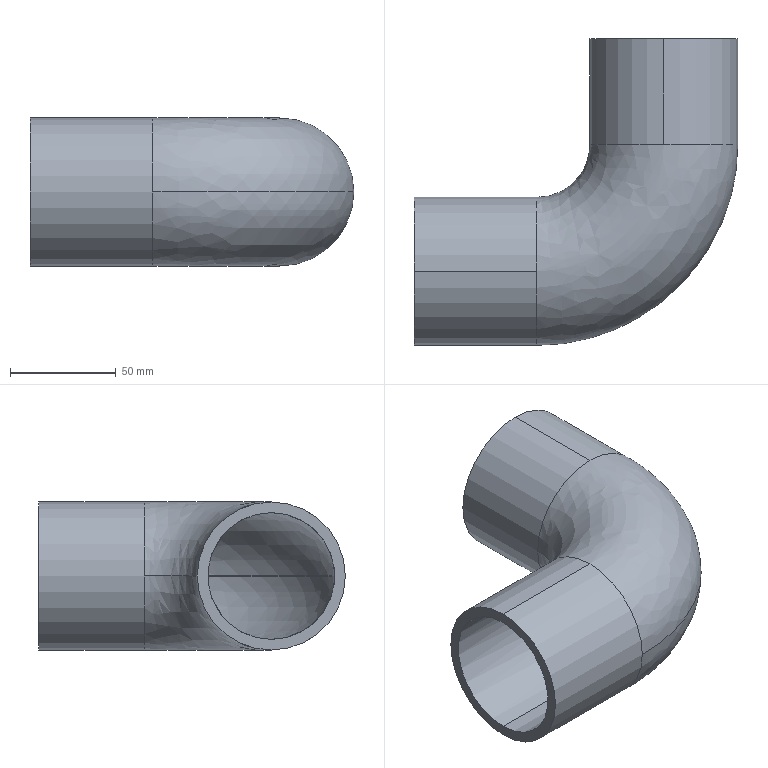Part | SolidWorks | features BaseBody 1 | 1 solid | 15 faces | box 153.045 x 145 x 70 mm | volume 206542 mm3 | cylinder 8 | spline 5 | plane 2 | commonest cylinder face diameters 60 x4 70 x4
STEP:
#1=CARTESIAN_POINT('',(58.045,0.,-35.));
#2=VERTEX_POINT('',#1);
#3=CARTESIAN_POINT('',(58.045,35.,-0.004506));
#4=VERTEX_POINT('',#3);
#5=CARTESIAN_POINT('',(58.045,0.,0.));
#6=DIRECTION('',(1.,0.,0.));
#7=DIRECTION('',(0.,-1.,0.));
#8=AXIS2_PLACEMENT_3D('',#5,#6,#7);
#9=CIRCLE('',#8,35.);
#10=EDGE_CURVE('',#2,#4,#9,.T.);
#11=ORIENTED_EDGE('',*,*,#10,.F.);
#12=CARTESIAN_POINT('',(0.,0.,-35.));
#13=VERTEX_POINT('',#12);
#14=CARTESIAN_POINT('',(58.045,0.,-35.));
#15=DIRECTION('',(-1.,0.,0.));
#16=VECTOR('',#15,1000.);
#17=LINE('',#14,#16);
#18=EDGE_CURVE('',#2,#13,#17,.T.);
#19=ORIENTED_EDGE('',*,*,#18,.T.);
#20=CARTESIAN_POINT('',(0.,0.,35.));
#21=VERTEX_POINT('',#20);
#22=CARTESIAN_POINT('',(0.,0.,0.));
#23=DIRECTION('',(1.,0.,0.));
#24=DIRECTION('',(0.,0.,1.));
#25=AXIS2_PLACEMENT_3D('',#22,#23,#24);
#26=CIRCLE('',#25,35.);
#27=EDGE_CURVE('',#13,#21,#26,.T.);
#28=ORIENTED_EDGE('',*,*,#27,.T.);
#29=CARTESIAN_POINT('',(58.045,0.,35.));
#30=VERTEX_POINT('',#29);
#31=CARTESIAN_POINT('',(58.045,0.,35.));
#32=DIRECTION('',(-1.,0.,0.));
#33=VECTOR('',#32,1000.);
#34=LINE('',#31,#33);
#35=EDGE_CURVE('',#30,#21,#34,.T.);
#36=ORIENTED_EDGE('',*,*,#35,.F.);
#37=CARTESIAN_POINT('',(58.045,0.,0.));
#38=DIRECTION('',(-1.,0.,0.));
#39=DIRECTION('',(0.,0.,1.));
#40=AXIS2_PLACEMENT_3D('',#37,#38,#39);
#41=CIRCLE('',#40,35.);
#42=EDGE_CURVE('',#30,#4,#41,.T.);
#43=ORIENTED_EDGE('',*,*,#42,.T.);
#44=EDGE_LOOP('',(#11,#19,#28,#36,#43));
#45=FACE_OUTER_BOUND('',#44,.T.);
#46=CARTESIAN_POINT('',(58.045,0.,0.));
#47=DIRECTION('',(-1.,0.,0.));
#48=DIRECTION('',(0.,0.,1.));
#49=AXIS2_PLACEMENT_3D('',#46,#47,#48);
#50=CYLINDRICAL_SURFACE('',#49,35.);
#51=ADVANCED_FACE('',(#45),#50,.T.);
#52=CARTESIAN_POINT('',(118.045,60.,-35.));
#53=VERTEX_POINT('',#52);
#54=CARTESIAN_POINT('',(153.045,60.,0.000000001));
#55=VERTEX_POINT('',#54);
#56=CARTESIAN_POINT('',(118.045,60.,0.));
#57=DIRECTION('',(0.,-1.,0.));
#58=DIRECTION('',(1.,0.,0.));
#59=AXIS2_PLACEMENT_3D('',#56,#57,#58);
#60=CIRCLE('',#59,35.);
#61=EDGE_CURVE('',#53,#55,#60,.T.);
#62=ORIENTED_EDGE('',*,*,#61,.F.);
#63=CARTESIAN_POINT('',(118.045,110.,-35.));
#64=VERTEX_POINT('',#63);
#65=CARTESIAN_POINT('',(118.045,60.,-35.));
#66=DIRECTION('',(0.,1.,0.));
#67=VECTOR('',#66,1000.);
#68=LINE('',#65,#67);
#69=EDGE_CURVE('',#53,#64,#68,.T.);
#70=ORIENTED_EDGE('',*,*,#69,.T.);
#71=CARTESIAN_POINT('',(118.045,110.,35.));
#72=VERTEX_POINT('',#71);
#73=CARTESIAN_POINT('',(118.045,110.,0.));
#74=DIRECTION('',(0.,-1.,0.));
#75=DIRECTION('',(0.,0.,1.));
#76=AXIS2_PLACEMENT_3D('',#73,#74,#75);
#77=CIRCLE('',#76,35.);
#78=EDGE_CURVE('',#64,#72,#77,.T.);
#79=ORIENTED_EDGE('',*,*,#78,.T.);
#80=CARTESIAN_POINT('',(118.045,60.,35.));
#81=VERTEX_POINT('',#80);
#82=CARTESIAN_POINT('',(118.045,60.,35.));
#83=DIRECTION('',(0.,1.,0.));
#84=VECTOR('',#83,1000.);
#85=LINE('',#82,#84);
#86=EDGE_CURVE('',#81,#72,#85,.T.);
#87=ORIENTED_EDGE('',*,*,#86,.F.);
#88=CARTESIAN_POINT('',(118.045,60.,0.000000001));
#89=DIRECTION('',(0.,-1.,0.));
#90=DIRECTION('',(1.,0.,0.));
#91=AXIS2_PLACEMENT_3D('',#88,#89,#90);
#92=CIRCLE('',#91,35.);
#93=EDGE_CURVE('',#55,#81,#92,.T.);
#94=ORIENTED_EDGE('',*,*,#93,.F.);
#95=EDGE_LOOP('',(#62,#70,#79,#87,#94));
#96=FACE_OUTER_BOUND('',#95,.T.);
#97=CARTESIAN_POINT('',(118.045,60.,0.));
#98=DIRECTION('',(0.,1.,0.));
#99=DIRECTION('',(0.,0.,1.));
#100=AXIS2_PLACEMENT_3D('',#97,#98,#99);
#101=CYLINDRICAL_SURFACE('',#100,35.);
#102=ADVANCED_FACE('',(#96),#101,.T.);
#103=CARTESIAN_POINT('',(58.045,0.,-30.));
#104=VERTEX_POINT('',#103);
#105=CARTESIAN_POINT('',(58.045,-30.,-0.000000002));
#106=VERTEX_POINT('',#105);
#107=CARTESIAN_POINT('',(58.045,0.,0.));
#108=DIRECTION('',(-1.,0.,0.));
#109=DIRECTION('',(0.,0.,1.));
#110=AXIS2_PLACEMENT_3D('',#107,#108,#109);
#111=CIRCLE('',#110,30.);
#112=EDGE_CURVE('',#104,#106,#111,.T.);
#113=ORIENTED_EDGE('',*,*,#112,.F.);
#114=CARTESIAN_POINT('',(0.,0.,-30.));
#115=VERTEX_POINT('',#114);
#116=CARTESIAN_POINT('',(58.045,0.,-30.));
#117=DIRECTION('',(-1.,0.,0.));
#118=VECTOR('',#117,1000.);
#119=LINE('',#116,#118);
#120=EDGE_CURVE('',#104,#115,#119,.T.);
#121=ORIENTED_EDGE('',*,*,#120,.T.);
#122=CARTESIAN_POINT('',(0.,0.,30.));
#123=VERTEX_POINT('',#122);
#124=CARTESIAN_POINT('',(0.,0.,0.));
#125=DIRECTION('',(-1.,0.,0.));
#126=DIRECTION('',(0.,0.,1.));
#127=AXIS2_PLACEMENT_3D('',#124,#125,#126);
#128=CIRCLE('',#127,30.);
#129=EDGE_CURVE('',#115,#123,#128,.T.);
#130=ORIENTED_EDGE('',*,*,#129,.T.);
#131=CARTESIAN_POINT('',(58.045,0.,30.));
#132=VERTEX_POINT('',#131);
#133=CARTESIAN_POINT('',(58.045,0.,30.));
#134=DIRECTION('',(-1.,0.,0.));
#135=VECTOR('',#134,1000.);
#136=LINE('',#133,#135);
#137=EDGE_CURVE('',#132,#123,#136,.T.);
#138=ORIENTED_EDGE('',*,*,#137,.F.);
#139=CARTESIAN_POINT('',(58.045,-30.,0.0003745));
#140=VERTEX_POINT('',#139);
#141=CARTESIAN_POINT('',(58.045,0.,0.));
#142=DIRECTION('',(-1.,0.,0.));
#143=DIRECTION('',(0.,0.,1.));
#144=AXIS2_PLACEMENT_3D('',#141,#142,#143);
#145=CIRCLE('',#144,30.);
#146=EDGE_CURVE('',#140,#132,#145,.T.);
#147=ORIENTED_EDGE('',*,*,#146,.F.);
#148=CARTESIAN_POINT('',(58.045,0.,0.));
#149=DIRECTION('',(-1.,0.,0.));
#150=DIRECTION('',(0.,0.,1.));
#151=AXIS2_PLACEMENT_3D('',#148,#149,#150);
#152=CIRCLE('',#151,30.);
#153=EDGE_CURVE('',#106,#140,#152,.T.);
#154=ORIENTED_EDGE('',*,*,#153,.F.);
#155=EDGE_LOOP('',(#113,#121,#130,#138,#147,#154));
#156=FACE_OUTER_BOUND('',#155,.T.);
#157=CARTESIAN_POINT('',(58.045,0.,0.));
#158=DIRECTION('',(-1.,0.,0.));
#159=DIRECTION('',(0.,0.,1.));
#160=AXIS2_PLACEMENT_3D('',#157,#158,#159);
#161=CYLINDRICAL_SURFACE('',#160,30.);
#162=ADVANCED_FACE('',(#156),#161,.F.);
#163=CARTESIAN_POINT('',(118.045,60.,-30.));
#164=VERTEX_POINT('',#163);
#165=CARTESIAN_POINT('',(88.045,60.,-0.000000012));
#166=VERTEX_POINT('',#165);
#167=CARTESIAN_POINT('',(118.045,60.,0.));
#168=DIRECTION('',(0.,1.,0.));
#169=DIRECTION('',(0.,0.,1.));
#170=AXIS2_PLACEMENT_3D('',#167,#168,#169);
#171=CIRCLE('',#170,30.);
#172=EDGE_CURVE('',#164,#166,#171,.T.);
#173=ORIENTED_EDGE('',*,*,#172,.F.);
#174=CARTESIAN_POINT('',(118.045,110.,-30.));
#175=VERTEX_POINT('',#174);
#176=CARTESIAN_POINT('',(118.045,60.,-30.));
#177=DIRECTION('',(0.,1.,0.));
#178=VECTOR('',#177,1000.);
#179=LINE('',#176,#178);
#180=EDGE_CURVE('',#164,#175,#179,.T.);
#181=ORIENTED_EDGE('',*,*,#180,.T.);
#182=CARTESIAN_POINT('',(118.045,110.,30.));
#183=VERTEX_POINT('',#182);
#184=CARTESIAN_POINT('',(118.045,110.,0.));
#185=DIRECTION('',(0.,-1.,0.));
#186=DIRECTION('',(0.,0.,1.));
#187=AXIS2_PLACEMENT_3D('',#184,#185,#186);
#188=CIRCLE('',#187,30.);
#189=EDGE_CURVE('',#183,#175,#188,.T.);
#190=ORIENTED_EDGE('',*,*,#189,.F.);
#191=CARTESIAN_POINT('',(118.045,60.,30.));
#192=VERTEX_POINT('',#191);
#193=CARTESIAN_POINT('',(118.045,60.,30.));
#194=DIRECTION('',(0.,1.,0.));
#195=VECTOR('',#194,1000.);
#196=LINE('',#193,#195);
#197=EDGE_CURVE('',#192,#183,#196,.T.);
#198=ORIENTED_EDGE('',*,*,#197,.F.);
#199=CARTESIAN_POINT('',(118.045,60.,0.));
#200=DIRECTION('',(0.,1.,0.));
#201=DIRECTION('',(0.,0.,1.));
#202=AXIS2_PLACEMENT_3D('',#199,#200,#201);
#203=CIRCLE('',#202,30.);
#204=EDGE_CURVE('',#166,#192,#203,.T.);
#205=ORIENTED_EDGE('',*,*,#204,.F.);
#206=EDGE_LOOP('',(#173,#181,#190,#198,#205));
#207=FACE_OUTER_BOUND('',#206,.T.);
#208=CARTESIAN_POINT('',(118.045,60.,0.));
#209=DIRECTION('',(0.,1.,0.));
#210=DIRECTION('',(0.,0.,1.));
#211=AXIS2_PLACEMENT_3D('',#208,#209,#210);
#212=CYLINDRICAL_SURFACE('',#211,30.);
#213=ADVANCED_FACE('',(#207),#212,.F.);
#214=CARTESIAN_POINT('',(58.045,30.,-0.000000006));
#215=VERTEX_POINT('',#214);
#216=CARTESIAN_POINT('',(58.045,0.,0.));
#217=DIRECTION('',(-1.,0.,0.));
#218=DIRECTION('',(0.,0.,1.));
#219=AXIS2_PLACEMENT_3D('',#216,#217,#218);
#220=CIRCLE('',#219,30.);
#221=EDGE_CURVE('',#215,#104,#220,.T.);
#222=ORIENTED_EDGE('',*,*,#221,.T.);
#223=ORIENTED_EDGE('',*,*,#112,.T.);
#224=CARTESIAN_POINT('',(148.045,60.,-0.000000002));
#225=VERTEX_POINT('',#224);
#226=CARTESIAN_POINT('',(58.045,60.,-0.000000004));
#227=DIRECTION('',(0.,0.,1.));
#228=DIRECTION('',(0.,-1.,0.));
#229=AXIS2_PLACEMENT_3D('',#226,#227,#228);
#230=CIRCLE('',#229,90.);
#231=EDGE_CURVE('',#106,#225,#230,.T.);
#232=ORIENTED_EDGE('',*,*,#231,.T.);
#233=CARTESIAN_POINT('',(118.045,60.,0.));
#234=DIRECTION('',(0.,1.,0.));
#235=DIRECTION('',(0.,0.,1.));
#236=AXIS2_PLACEMENT_3D('',#233,#234,#235);
#237=CIRCLE('',#236,30.);
#238=EDGE_CURVE('',#225,#164,#237,.T.);
#239=ORIENTED_EDGE('',*,*,#238,.T.);
#240=ORIENTED_EDGE('',*,*,#172,.T.);
#241=CARTESIAN_POINT('',(58.045,30.,-0.000000006));
#242=CARTESIAN_POINT('',(60.009,30.,-0.0002528));
#243=CARTESIAN_POINT('',(61.972,30.193,-0.000474));
#244=CARTESIAN_POINT('',(65.823,30.96,-0.0008532));
#245=CARTESIAN_POINT('',(67.711,31.532,-0.001011));
#246=CARTESIAN_POINT('',(71.34,33.035,-0.001264));
#247=CARTESIAN_POINT('',(73.08,33.965,-0.001359));
#248=CARTESIAN_POINT('',(76.345,36.147,-0.001485));
#249=CARTESIAN_POINT('',(77.87,37.398,-0.001517));
#250=CARTESIAN_POINT('',(80.647,40.175,-0.001517));
#251=CARTESIAN_POINT('',(81.898,41.7,-0.001485));
#252=CARTESIAN_POINT('',(84.08,44.965,-0.001359));
#253=CARTESIAN_POINT('',(85.01,46.705,-0.001264));
#254=CARTESIAN_POINT('',(86.513,50.334,-0.001011));
#255=CARTESIAN_POINT('',(87.086,52.222,-0.0008532));
#256=CARTESIAN_POINT('',(87.852,56.073,-0.000474));
#257=CARTESIAN_POINT('',(88.045,58.037,-0.0002528));
#258=CARTESIAN_POINT('',(88.045,60.,-0.000000012));
#259=B_SPLINE_CURVE_WITH_KNOTS('',3,(#241,#242,#243,#244,#245,#246,#247,#248,#249,#250,#251,#252,#253,#254,#255,#256,#257,#258),.UNSPECIFIED.,.F.,.F.,(4,2,2,2,2,2,2,2,4),(0.,0.125,0.25,0.375,0.5,0.625,0.75,0.875,1.),.UNSPECIFIED.);
#260=EDGE_CURVE('',#215,#166,#259,.T.);
#261=ORIENTED_EDGE('',*,*,#260,.F.);
#262=EDGE_LOOP('',(#222,#223,#232,#239,#240,#261));
#263=FACE_OUTER_BOUND('',#262,.T.);
#264=CARTESIAN_POINT('',(58.045,-30.,-0.000000002));
#265=CARTESIAN_POINT('',(110.766,-30.,-0.000000001));
#266=CARTESIAN_POINT('',(148.045,7.279,-0.000000001));
#267=CARTESIAN_POINT('',(148.045,60.,-0.000000002));
#268=CARTESIAN_POINT('',(58.045,-30.,-17.705));
#269=CARTESIAN_POINT('',(110.766,-30.,-17.705));
#270=CARTESIAN_POINT('',(148.045,7.279,-17.705));
#271=CARTESIAN_POINT('',(148.045,60.,-17.705));
#272=CARTESIAN_POINT('',(58.045,-17.422,-30.166));
#273=CARTESIAN_POINT('',(103.398,-17.422,-30.166));
#274=CARTESIAN_POINT('',(135.467,14.647,-30.166));
#275=CARTESIAN_POINT('',(135.467,60.,-30.166));
#276=CARTESIAN_POINT('',(58.045,0.2827,-29.999));
#277=CARTESIAN_POINT('',(93.027,0.2827,-29.999));
#278=CARTESIAN_POINT('',(117.762,25.018,-29.999));
#279=CARTESIAN_POINT('',(117.762,60.,-29.999));
#280=CARTESIAN_POINT('',(58.045,17.987,-29.832));
#281=CARTESIAN_POINT('',(82.656,17.987,-29.832));
#282=CARTESIAN_POINT('',(100.058,35.389,-29.832));
#283=CARTESIAN_POINT('',(100.058,60.,-29.832));
#284=CARTESIAN_POINT('',(58.045,30.328,-17.137));
#285=CARTESIAN_POINT('',(75.426,30.328,-17.137));
#286=CARTESIAN_POINT('',(87.717,42.619,-17.137));
#287=CARTESIAN_POINT('',(87.717,60.,-17.137));
#288=CARTESIAN_POINT('',(58.045,29.995,0.5655));
#289=CARTESIAN_POINT('',(75.622,29.995,0.5655));
#290=CARTESIAN_POINT('',(88.05,42.423,0.5655));
#291=CARTESIAN_POINT('',(88.05,60.,0.5655));
#292=(BOUNDED_SURFACE()B_SPLINE_SURFACE(3,3,((#264,#265,#266,#267),(#268,#269,#270,#271),(#272,#273,#274,#275),(#276,#277,#278,#279),(#280,#281,#282,#283),(#284,#285,#286,#287),(#288,#289,#290,#291)),.UNSPECIFIED.,.F.,.F.,.F.)B_SPLINE_SURFACE_WITH_KNOTS((4,3,4),(4,4),(0.,0.5,1.),(0.,1.),.UNSPECIFIED.)GEOMETRIC_REPRESENTATION_ITEM()RATIONAL_B_SPLINE_SURFACE(((1.,0.8047,0.8047,1.),(0.8025,0.6458,0.6458,0.8025),(0.8025,0.6458,0.6458,0.8025),(1.,0.8047,0.8047,1.),(0.8025,0.6458,0.6458,0.8025),(0.8025,0.6458,0.6458,0.8025),(1.,0.8047,0.8047,1.)))REPRESENTATION_ITEM('')SURFACE());
#293=ADVANCED_FACE('',(#263),#292,.F.);
#294=CARTESIAN_POINT('',(58.045,-35.,0.000000001));
#295=VERTEX_POINT('',#294);
#296=CARTESIAN_POINT('',(58.045,0.,0.));
#297=DIRECTION('',(1.,0.,0.));
#298=DIRECTION('',(0.,-1.,0.));
#299=AXIS2_PLACEMENT_3D('',#296,#297,#298);
#300=CIRCLE('',#299,35.);
#301=EDGE_CURVE('',#295,#2,#300,.T.);
#302=ORIENTED_EDGE('',*,*,#301,.T.);
#303=ORIENTED_EDGE('',*,*,#10,.T.);
#304=CARTESIAN_POINT('',(83.045,60.,0.004506));
#305=VERTEX_POINT('',#304);
#306=CARTESIAN_POINT('',(58.045,35.,-0.004506));
#307=CARTESIAN_POINT('',(60.128,35.,-0.003755));
#308=CARTESIAN_POINT('',(62.154,35.261,-0.003051));
#309=CARTESIAN_POINT('',(65.981,36.211,-0.001737));
#310=CARTESIAN_POINT('',(67.782,36.899,-0.001127));
#311=CARTESIAN_POINT('',(71.093,38.594,-0.000000008));
#312=CARTESIAN_POINT('',(72.603,39.601,0.0005164));
#313=CARTESIAN_POINT('',(75.3,41.825,0.001455));
#314=CARTESIAN_POINT('',(76.488,43.043,0.001878));
#315=CARTESIAN_POINT('',(78.541,45.591,0.002629));
#316=CARTESIAN_POINT('',(79.406,46.922,0.002957));
#317=CARTESIAN_POINT('',(80.837,49.615,0.003521));
#318=CARTESIAN_POINT('',(81.402,50.976,0.003755));
#319=CARTESIAN_POINT('',(82.27,53.665,0.004131));
#320=CARTESIAN_POINT('',(82.573,54.992,0.004272));
#321=CARTESIAN_POINT('',(82.96,57.565,0.004459));
#322=CARTESIAN_POINT('',(83.045,58.811,0.004506));
#323=CARTESIAN_POINT('',(83.045,60.,0.004506));
#324=B_SPLINE_CURVE_WITH_KNOTS('',3,(#306,#307,#308,#309,#310,#311,#312,#313,#314,#315,#316,#317,#318,#319,#320,#321,#322,#323),.UNSPECIFIED.,.F.,.F.,(4,2,2,2,2,2,2,2,4),(0.,0.125,0.25,0.375,0.5,0.625,0.75,0.875,1.),.UNSPECIFIED.);
#325=EDGE_CURVE('',#4,#305,#324,.T.);
#326=ORIENTED_EDGE('',*,*,#325,.T.);
#327=CARTESIAN_POINT('',(118.045,60.,0.));
#328=DIRECTION('',(0.,-1.,0.));
#329=DIRECTION('',(1.,0.,0.));
#330=AXIS2_PLACEMENT_3D('',#327,#328,#329);
#331=CIRCLE('',#330,35.);
#332=EDGE_CURVE('',#305,#53,#331,.T.);
#333=ORIENTED_EDGE('',*,*,#332,.T.);
#334=ORIENTED_EDGE('',*,*,#61,.T.);
#335=CARTESIAN_POINT('',(58.045,60.,-0.000000001));
#336=DIRECTION('',(0.,0.,-1.));
#337=DIRECTION('',(0.,-1.,0.));
#338=AXIS2_PLACEMENT_3D('',#335,#336,#337);
#339=CIRCLE('',#338,95.);
#340=EDGE_CURVE('',#55,#295,#339,.T.);
#341=ORIENTED_EDGE('',*,*,#340,.T.);
#342=EDGE_LOOP('',(#302,#303,#326,#333,#334,#341));
#343=FACE_OUTER_BOUND('',#342,.T.);
#344=CARTESIAN_POINT('',(58.045,-35.,0.000000001));
#345=CARTESIAN_POINT('',(113.695,-35.,0.000000002));
#346=CARTESIAN_POINT('',(153.045,4.35,0.000000002));
#347=CARTESIAN_POINT('',(153.045,60.,0.000000001));
#348=CARTESIAN_POINT('',(58.045,-35.,-20.657));
#349=CARTESIAN_POINT('',(113.695,-35.,-20.657));
#350=CARTESIAN_POINT('',(153.045,4.35,-20.657));
#351=CARTESIAN_POINT('',(153.045,60.,-20.657));
#352=CARTESIAN_POINT('',(58.045,-20.324,-35.194));
#353=CARTESIAN_POINT('',(105.098,-20.324,-35.194));
#354=CARTESIAN_POINT('',(138.369,12.947,-35.194));
#355=CARTESIAN_POINT('',(138.369,60.,-35.194));
#356=CARTESIAN_POINT('',(58.045,0.3321,-34.998));
#357=CARTESIAN_POINT('',(92.998,0.3321,-34.998));
#358=CARTESIAN_POINT('',(117.713,25.047,-34.998));
#359=CARTESIAN_POINT('',(117.713,60.,-34.998));
#360=CARTESIAN_POINT('',(58.045,20.988,-34.802));
#361=CARTESIAN_POINT('',(80.898,20.988,-34.802));
#362=CARTESIAN_POINT('',(97.057,37.147,-34.802));
#363=CARTESIAN_POINT('',(97.057,60.,-34.802));
#364=CARTESIAN_POINT('',(58.045,35.386,-19.989));
#365=CARTESIAN_POINT('',(72.464,35.386,-19.989));
#366=CARTESIAN_POINT('',(82.659,45.581,-19.989));
#367=CARTESIAN_POINT('',(82.659,60.,-19.989));
#368=CARTESIAN_POINT('',(58.045,34.994,0.6642));
#369=CARTESIAN_POINT('',(72.693,34.994,0.6642));
#370=CARTESIAN_POINT('',(83.051,45.352,0.6642));
#371=CARTESIAN_POINT('',(83.051,60.,0.6642));
#372=(BOUNDED_SURFACE()B_SPLINE_SURFACE(3,3,((#344,#345,#346,#347),(#348,#349,#350,#351),(#352,#353,#354,#355),(#356,#357,#358,#359),(#360,#361,#362,#363),(#364,#365,#366,#367),(#368,#369,#370,#371)),.UNSPECIFIED.,.F.,.F.,.F.)B_SPLINE_SURFACE_WITH_KNOTS((4,3,4),(4,4),(0.,0.5,1.),(0.,1.),.UNSPECIFIED.)GEOMETRIC_REPRESENTATION_ITEM()RATIONAL_B_SPLINE_SURFACE(((1.,0.8047,0.8047,1.),(0.8025,0.6458,0.6458,0.8025),(0.8025,0.6458,0.6458,0.8025),(1.,0.8047,0.8047,1.),(0.8025,0.6458,0.6458,0.8025),(0.8025,0.6458,0.6458,0.8025),(1.,0.8047,0.8047,1.)))REPRESENTATION_ITEM('')SURFACE());
#373=ADVANCED_FACE('',(#343),#372,.T.);
#374=ORIENTED_EDGE('',*,*,#18,.F.);
#375=ORIENTED_EDGE('',*,*,#301,.F.);
#376=CARTESIAN_POINT('',(58.045,0.,0.));
#377=DIRECTION('',(-1.,0.,0.));
#378=DIRECTION('',(0.,0.,1.));
#379=AXIS2_PLACEMENT_3D('',#376,#377,#378);
#380=CIRCLE('',#379,35.);
#381=EDGE_CURVE('',#295,#30,#380,.T.);
#382=ORIENTED_EDGE('',*,*,#381,.T.);
#383=ORIENTED_EDGE('',*,*,#35,.T.);
#384=CARTESIAN_POINT('',(0.,0.,0.));
#385=DIRECTION('',(1.,0.,0.));
#386=DIRECTION('',(0.,0.,1.));
#387=AXIS2_PLACEMENT_3D('',#384,#385,#386);
#388=CIRCLE('',#387,35.);
#389=EDGE_CURVE('',#21,#13,#388,.T.);
#390=ORIENTED_EDGE('',*,*,#389,.T.);
#391=EDGE_LOOP('',(#374,#375,#382,#383,#390));
#392=FACE_OUTER_BOUND('',#391,.T.);
#393=CARTESIAN_POINT('',(58.045,0.,0.));
#394=DIRECTION('',(-1.,0.,0.));
#395=DIRECTION('',(0.,0.,1.));
#396=AXIS2_PLACEMENT_3D('',#393,#394,#395);
#397=CYLINDRICAL_SURFACE('',#396,35.);
#398=ADVANCED_FACE('',(#392),#397,.T.);
#399=ORIENTED_EDGE('',*,*,#381,.F.);
#400=ORIENTED_EDGE('',*,*,#340,.F.);
#401=ORIENTED_EDGE('',*,*,#93,.T.);
#402=CARTESIAN_POINT('',(118.045,60.,0.000000001));
#403=DIRECTION('',(0.,-1.,0.));
#404=DIRECTION('',(1.,0.,0.));
#405=AXIS2_PLACEMENT_3D('',#402,#403,#404);
#406=CIRCLE('',#405,35.);
#407=EDGE_CURVE('',#81,#305,#406,.T.);
#408=ORIENTED_EDGE('',*,*,#407,.T.);
#409=ORIENTED_EDGE('',*,*,#325,.F.);
#410=ORIENTED_EDGE('',*,*,#42,.F.);
#411=EDGE_LOOP('',(#399,#400,#401,#408,#409,#410));
#412=FACE_OUTER_BOUND('',#411,.T.);
#413=CARTESIAN_POINT('',(58.045,34.994,-0.6642));
#414=CARTESIAN_POINT('',(72.693,34.994,-0.6642));
#415=CARTESIAN_POINT('',(83.051,45.352,-0.6642));
#416=CARTESIAN_POINT('',(83.051,60.,-0.6642));
#417=CARTESIAN_POINT('',(58.045,35.386,19.989));
#418=CARTESIAN_POINT('',(72.464,35.386,19.989));
#419=CARTESIAN_POINT('',(82.659,45.581,19.989));
#420=CARTESIAN_POINT('',(82.659,60.,19.989));
#421=CARTESIAN_POINT('',(58.045,20.988,34.802));
#422=CARTESIAN_POINT('',(80.898,20.988,34.802));
#423=CARTESIAN_POINT('',(97.057,37.147,34.802));
#424=CARTESIAN_POINT('',(97.057,60.,34.802));
#425=CARTESIAN_POINT('',(58.045,0.3321,34.998));
#426=CARTESIAN_POINT('',(92.998,0.3321,34.998));
#427=CARTESIAN_POINT('',(117.713,25.047,34.998));
#428=CARTESIAN_POINT('',(117.713,60.,34.998));
#429=CARTESIAN_POINT('',(58.045,-20.324,35.194));
#430=CARTESIAN_POINT('',(105.098,-20.324,35.194));
#431=CARTESIAN_POINT('',(138.369,12.947,35.194));
#432=CARTESIAN_POINT('',(138.369,60.,35.194));
#433=CARTESIAN_POINT('',(58.045,-35.,20.657));
#434=CARTESIAN_POINT('',(113.695,-35.,20.657));
#435=CARTESIAN_POINT('',(153.045,4.35,20.657));
#436=CARTESIAN_POINT('',(153.045,60.,20.657));
#437=CARTESIAN_POINT('',(58.045,-35.,0.000000001));
#438=CARTESIAN_POINT('',(113.695,-35.,0.));
#439=CARTESIAN_POINT('',(153.045,4.35,0.));
#440=CARTESIAN_POINT('',(153.045,60.,0.000000001));
#441=(BOUNDED_SURFACE()B_SPLINE_SURFACE(3,3,((#413,#414,#415,#416),(#417,#418,#419,#420),(#421,#422,#423,#424),(#425,#426,#427,#428),(#429,#430,#431,#432),(#433,#434,#435,#436),(#437,#438,#439,#440)),.UNSPECIFIED.,.F.,.F.,.T.)B_SPLINE_SURFACE_WITH_KNOTS((4,3,4),(4,4),(0.,0.5,1.),(0.,1.),.UNSPECIFIED.)GEOMETRIC_REPRESENTATION_ITEM()RATIONAL_B_SPLINE_SURFACE(((1.,0.8047,0.8047,1.),(0.8025,0.6458,0.6458,0.8025),(0.8025,0.6458,0.6458,0.8025),(1.,0.8047,0.8047,1.),(0.8025,0.6458,0.6458,0.8025),(0.8025,0.6458,0.6458,0.8025),(1.,0.8047,0.8047,1.)))REPRESENTATION_ITEM('')SURFACE());
#442=ADVANCED_FACE('',(#412),#441,.T.);
#443=ORIENTED_EDGE('',*,*,#69,.F.);
#444=ORIENTED_EDGE('',*,*,#332,.F.);
#445=ORIENTED_EDGE('',*,*,#407,.F.);
#446=ORIENTED_EDGE('',*,*,#86,.T.);
#447=CARTESIAN_POINT('',(118.045,110.,0.));
#448=DIRECTION('',(0.,-1.,0.));
#449=DIRECTION('',(0.,0.,1.));
#450=AXIS2_PLACEMENT_3D('',#447,#448,#449);
#451=CIRCLE('',#450,35.);
#452=EDGE_CURVE('',#72,#64,#451,.T.);
#453=ORIENTED_EDGE('',*,*,#452,.T.);
#454=EDGE_LOOP('',(#443,#444,#445,#446,#453));
#455=FACE_OUTER_BOUND('',#454,.T.);
#456=CARTESIAN_POINT('',(118.045,60.,0.));
#457=DIRECTION('',(0.,1.,0.));
#458=DIRECTION('',(0.,0.,1.));
#459=AXIS2_PLACEMENT_3D('',#456,#457,#458);
#460=CYLINDRICAL_SURFACE('',#459,35.);
#461=ADVANCED_FACE('',(#455),#460,.T.);
#462=CARTESIAN_POINT('',(0.,0.,0.));
#463=DIRECTION('',(-1.,0.,0.));
#464=DIRECTION('',(0.,0.,1.));
#465=AXIS2_PLACEMENT_3D('',#462,#463,#464);
#466=CIRCLE('',#465,30.);
#467=EDGE_CURVE('',#123,#115,#466,.T.);
#468=ORIENTED_EDGE('',*,*,#467,.F.);
#469=ORIENTED_EDGE('',*,*,#129,.F.);
#470=EDGE_LOOP('',(#468,#469));
#471=FACE_BOUND('',#470,.T.);
#472=ORIENTED_EDGE('',*,*,#389,.F.);
#473=ORIENTED_EDGE('',*,*,#27,.F.);
#474=EDGE_LOOP('',(#472,#473));
#475=FACE_OUTER_BOUND('',#474,.T.);
#476=CARTESIAN_POINT('',(0.,0.,0.));
#477=DIRECTION('',(1.,0.,0.));
#478=DIRECTION('',(0.,0.,-1.));
#479=AXIS2_PLACEMENT_3D('',#476,#477,#478);
#480=PLANE('',#479);
#481=ADVANCED_FACE('',(#471,#475),#480,.F.);
#482=ORIENTED_EDGE('',*,*,#189,.T.);
#483=CARTESIAN_POINT('',(118.045,110.,0.));
#484=DIRECTION('',(0.,-1.,0.));
#485=DIRECTION('',(0.,0.,1.));
#486=AXIS2_PLACEMENT_3D('',#483,#484,#485);
#487=CIRCLE('',#486,30.);
#488=EDGE_CURVE('',#175,#183,#487,.T.);
#489=ORIENTED_EDGE('',*,*,#488,.T.);
#490=EDGE_LOOP('',(#482,#489));
#491=FACE_BOUND('',#490,.T.);
#492=ORIENTED_EDGE('',*,*,#452,.F.);
#493=ORIENTED_EDGE('',*,*,#78,.F.);
#494=EDGE_LOOP('',(#492,#493));
#495=FACE_OUTER_BOUND('',#494,.T.);
#496=CARTESIAN_POINT('',(118.045,110.,0.));
#497=DIRECTION('',(0.,1.,0.));
#498=DIRECTION('',(0.,0.,1.));
#499=AXIS2_PLACEMENT_3D('',#496,#497,#498);
#500=PLANE('',#499);
#501=ADVANCED_FACE('',(#491,#495),#500,.T.);
#502=ORIENTED_EDGE('',*,*,#120,.F.);
#503=ORIENTED_EDGE('',*,*,#221,.F.);
#504=CARTESIAN_POINT('',(58.045,0.,0.));
#505=DIRECTION('',(-1.,0.,0.));
#506=DIRECTION('',(0.,0.,1.));
#507=AXIS2_PLACEMENT_3D('',#504,#505,#506);
#508=CIRCLE('',#507,30.);
#509=EDGE_CURVE('',#132,#215,#508,.T.);
#510=ORIENTED_EDGE('',*,*,#509,.F.);
#511=ORIENTED_EDGE('',*,*,#137,.T.);
#512=ORIENTED_EDGE('',*,*,#467,.T.);
#513=EDGE_LOOP('',(#502,#503,#510,#511,#512));
#514=FACE_OUTER_BOUND('',#513,.T.);
#515=CARTESIAN_POINT('',(58.045,0.,0.));
#516=DIRECTION('',(-1.,0.,0.));
#517=DIRECTION('',(0.,0.,1.));
#518=AXIS2_PLACEMENT_3D('',#515,#516,#517);
#519=CYLINDRICAL_SURFACE('',#518,30.);
#520=ADVANCED_FACE('',(#514),#519,.F.);
#521=ORIENTED_EDGE('',*,*,#180,.F.);
#522=ORIENTED_EDGE('',*,*,#238,.F.);
#523=CARTESIAN_POINT('',(148.045,60.,0.0003745));
#524=VERTEX_POINT('',#523);
#525=CARTESIAN_POINT('',(118.045,60.,0.));
#526=DIRECTION('',(0.,1.,0.));
#527=DIRECTION('',(0.,0.,1.));
#528=AXIS2_PLACEMENT_3D('',#525,#526,#527);
#529=CIRCLE('',#528,30.);
#530=EDGE_CURVE('',#524,#225,#529,.T.);
#531=ORIENTED_EDGE('',*,*,#530,.F.);
#532=CARTESIAN_POINT('',(118.045,60.,0.));
#533=DIRECTION('',(0.,1.,0.));
#534=DIRECTION('',(0.,0.,1.));
#535=AXIS2_PLACEMENT_3D('',#532,#533,#534);
#536=CIRCLE('',#535,30.);
#537=EDGE_CURVE('',#192,#524,#536,.T.);
#538=ORIENTED_EDGE('',*,*,#537,.F.);
#539=ORIENTED_EDGE('',*,*,#197,.T.);
#540=ORIENTED_EDGE('',*,*,#488,.F.);
#541=EDGE_LOOP('',(#521,#522,#531,#538,#539,#540));
#542=FACE_OUTER_BOUND('',#541,.T.);
#543=CARTESIAN_POINT('',(118.045,60.,0.));
#544=DIRECTION('',(0.,1.,0.));
#545=DIRECTION('',(0.,0.,1.));
#546=AXIS2_PLACEMENT_3D('',#543,#544,#545);
#547=CYLINDRICAL_SURFACE('',#546,30.);
#548=ADVANCED_FACE('',(#542),#547,.F.);
#549=ORIENTED_EDGE('',*,*,#231,.F.);
#550=ORIENTED_EDGE('',*,*,#153,.T.);
#551=CARTESIAN_POINT('',(58.045,60.,0.0003745));
#552=DIRECTION('',(0.,0.,-1.));
#553=DIRECTION('',(0.,-1.,0.));
#554=AXIS2_PLACEMENT_3D('',#551,#552,#553);
#555=CIRCLE('',#554,90.);
#556=EDGE_CURVE('',#524,#140,#555,.T.);
#557=ORIENTED_EDGE('',*,*,#556,.F.);
#558=ORIENTED_EDGE('',*,*,#530,.T.);
#559=EDGE_LOOP('',(#549,#550,#557,#558));
#560=FACE_OUTER_BOUND('',#559,.T.);
#561=CARTESIAN_POINT('',(58.045,-30.,0.0003745));
#562=CARTESIAN_POINT('',(110.766,-30.,0.0003745));
#563=CARTESIAN_POINT('',(148.045,7.279,0.0003745));
#564=CARTESIAN_POINT('',(148.045,60.,0.0003745));
#565=CARTESIAN_POINT('',(58.045,-30.,0.0002497));
#566=CARTESIAN_POINT('',(110.766,-30.,0.0002497));
#567=CARTESIAN_POINT('',(148.045,7.279,0.0002497));
#568=CARTESIAN_POINT('',(148.045,60.,0.0002497));
#569=CARTESIAN_POINT('',(58.045,-30.,0.0001248));
#570=CARTESIAN_POINT('',(110.766,-30.,0.0001248));
#571=CARTESIAN_POINT('',(148.045,7.279,0.0001248));
#572=CARTESIAN_POINT('',(148.045,60.,0.0001248));
#573=CARTESIAN_POINT('',(58.045,-30.,-0.000000002));
#574=CARTESIAN_POINT('',(110.766,-30.,-0.000000001));
#575=CARTESIAN_POINT('',(148.045,7.279,-0.000000001));
#576=CARTESIAN_POINT('',(148.045,60.,-0.000000002));
#577=(BOUNDED_SURFACE()B_SPLINE_SURFACE(3,3,((#561,#562,#563,#564),(#565,#566,#567,#568),(#569,#570,#571,#572),(#573,#574,#575,#576)),.UNSPECIFIED.,.F.,.F.,.F.)B_SPLINE_SURFACE_WITH_KNOTS((4,4),(4,4),(0.,1.),(0.,1.),.UNSPECIFIED.)GEOMETRIC_REPRESENTATION_ITEM()RATIONAL_B_SPLINE_SURFACE(((1.,0.8047,0.8047,1.),(1.,0.8047,0.8047,1.),(1.,0.8047,0.8047,1.),(1.,0.8047,0.8047,1.)))REPRESENTATION_ITEM('')SURFACE());
#578=ADVANCED_FACE('',(#560),#577,.F.);
#579=ORIENTED_EDGE('',*,*,#260,.T.);
#580=ORIENTED_EDGE('',*,*,#204,.T.);
#581=ORIENTED_EDGE('',*,*,#537,.T.);
#582=ORIENTED_EDGE('',*,*,#556,.T.);
#583=ORIENTED_EDGE('',*,*,#146,.T.);
#584=ORIENTED_EDGE('',*,*,#509,.T.);
#585=EDGE_LOOP('',(#579,#580,#581,#582,#583,#584));
#586=FACE_OUTER_BOUND('',#585,.T.);
#587=CARTESIAN_POINT('',(58.045,29.995,-0.567));
#588=CARTESIAN_POINT('',(75.622,29.995,-0.567));
#589=CARTESIAN_POINT('',(88.05,42.423,-0.567));
#590=CARTESIAN_POINT('',(88.05,60.,-0.567));
#591=CARTESIAN_POINT('',(58.045,30.329,17.135));
#592=CARTESIAN_POINT('',(75.426,30.329,17.135));
#593=CARTESIAN_POINT('',(87.716,42.619,17.135));
#594=CARTESIAN_POINT('',(87.716,60.,17.135));
#595=CARTESIAN_POINT('',(58.045,17.988,29.831));
#596=CARTESIAN_POINT('',(82.655,17.988,29.831));
#597=CARTESIAN_POINT('',(100.057,35.39,29.831));
#598=CARTESIAN_POINT('',(100.057,60.,29.831));
#599=CARTESIAN_POINT('',(58.045,0.2837,29.999));
#600=CARTESIAN_POINT('',(93.026,0.2837,29.999));
#601=CARTESIAN_POINT('',(117.761,25.019,29.999));
#602=CARTESIAN_POINT('',(117.761,60.,29.999));
#603=CARTESIAN_POINT('',(58.045,-17.421,30.166));
#604=CARTESIAN_POINT('',(103.397,-17.421,30.166));
#605=CARTESIAN_POINT('',(135.466,14.648,30.166));
#606=CARTESIAN_POINT('',(135.466,60.,30.166));
#607=CARTESIAN_POINT('',(58.045,-30.,17.706));
#608=CARTESIAN_POINT('',(110.766,-30.,17.706));
#609=CARTESIAN_POINT('',(148.045,7.279,17.706));
#610=CARTESIAN_POINT('',(148.045,60.,17.706));
#611=CARTESIAN_POINT('',(58.045,-30.,0.0003745));
#612=CARTESIAN_POINT('',(110.766,-30.,0.0003745));
#613=CARTESIAN_POINT('',(148.045,7.279,0.0003745));
#614=CARTESIAN_POINT('',(148.045,60.,0.0003745));
#615=(BOUNDED_SURFACE()B_SPLINE_SURFACE(3,3,((#587,#588,#589,#590),(#591,#592,#593,#594),(#595,#596,#597,#598),(#599,#600,#601,#602),(#603,#604,#605,#606),(#607,#608,#609,#610),(#611,#612,#613,#614)),.UNSPECIFIED.,.F.,.F.,.T.)B_SPLINE_SURFACE_WITH_KNOTS((4,3,4),(4,4),(0.,0.5,1.),(0.,1.),.UNSPECIFIED.)GEOMETRIC_REPRESENTATION_ITEM()RATIONAL_B_SPLINE_SURFACE(((1.,0.8047,0.8047,1.),(0.8025,0.6458,0.6458,0.8025),(0.8025,0.6458,0.6458,0.8025),(1.,0.8047,0.8047,1.),(0.8025,0.6458,0.6458,0.8025),(0.8025,0.6458,0.6458,0.8025),(1.,0.8047,0.8047,1.)))REPRESENTATION_ITEM('')SURFACE());
#616=ADVANCED_FACE('',(#586),#615,.F.);
#617=CLOSED_SHELL('',(#51,#102,#162,#213,#293,#373,#398,#442,#461,#481,#501,#520,#548,#578,#616));
#618=MANIFOLD_SOLID_BREP('',#617);
#619=CARTESIAN_POINT('',(0.,0.,0.));
#620=DIRECTION('',(0.,0.,1.));
#621=DIRECTION('',(1.,0.,0.));
#622=AXIS2_PLACEMENT_3D('',#619,#620,#621);
#623=(LENGTH_UNIT()NAMED_UNIT(*)SI_UNIT(.MILLI.,.METRE.));
#624=UNCERTAINTY_MEASURE_WITH_UNIT(LENGTH_MEASURE(0.00001),#623,'','');
#625=(NAMED_UNIT(*)PLANE_ANGLE_UNIT()SI_UNIT($,.RADIAN.));
#626=(NAMED_UNIT(*)SI_UNIT($,.STERADIAN.)SOLID_ANGLE_UNIT());
#627=(GEOMETRIC_REPRESENTATION_CONTEXT(3)GLOBAL_UNCERTAINTY_ASSIGNED_CONTEXT((#624))GLOBAL_UNIT_ASSIGNED_CONTEXT((#623,#625,#626))REPRESENTATION_CONTEXT('',''));
#628=ADVANCED_BREP_SHAPE_REPRESENTATION('',(#618,#622),#627);